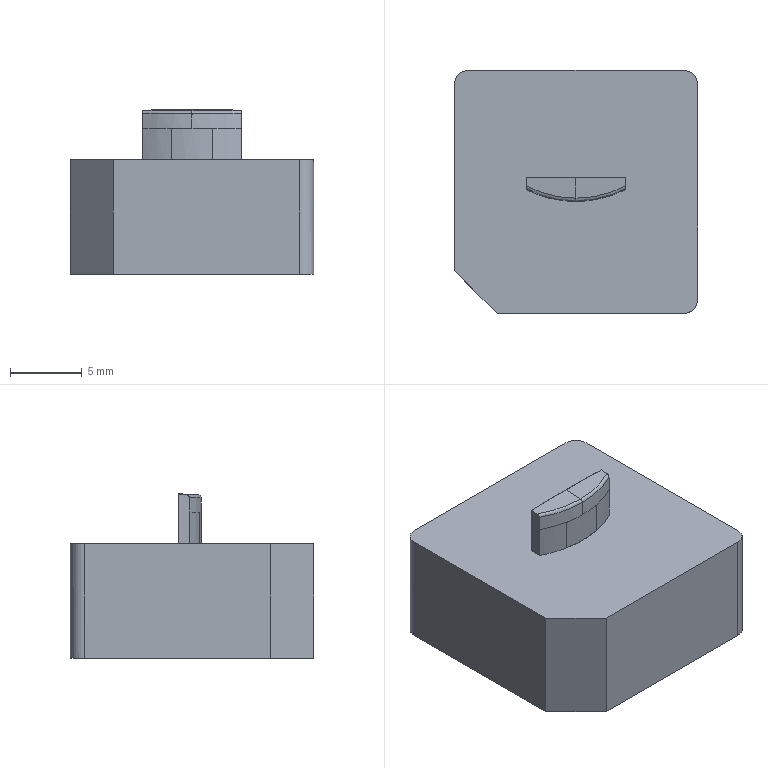CAM job | PowerMill | 3-axis milling, other | part box 17 x 17 x 11.498 mm
Tools:
number,name,type,diameter,tip_radius,length,cutting_length,overhang,flutes,holder,toolpaths_using
1,D10C,end_mill,10.0,0.0,60.0,,30.0,1,D42L35,1
2,D4C_1,end_mill,4.0,0.0,30.0,,4.0,1,D42L35,1
4,R1_1,ball_nosed,2.0,1.0,3.0,,2.0,1,D42L35,1
13,Text_D4_1,taper_spherical,4.0,0.3,60.0,,4.0,1,D42L35,1
1,D10C_1_1,end_mill,10.0,0.0,60.0,,11.96,1,D42L35,3
3,D10_1_1,end_mill,10.0,0.0,60.0,,11.64,1,D42L35,2
10,D3_1_1,end_mill,3.0,0.0,30.0,,3.76,1,D42L35,1
Operations:
program,toolpath,strategy,tool,tool_number,tool_diameter,tip_radius,flutes,spindle_rpm,feed_cut,surface_speed_m_min_computed,feed_per_tooth_computed,tolerance,thickness,stepover,stepdown,cut_length,cut_time_min,total_time_min,workplane
29-B01-8-F,精公开粗01-扫面平行-D10C,raster_area_clear,D10C_1_1,1,10.0,0.0,1.0,8000.0,10000.0,251.33,1.25,0.03,0.28,6.0,1.0,135.36,0.013,0.0178,
29-B01-8-F,精公开粗01-外形偏置-D10C,offset_area_clear,D10C_1_1,1,10.0,0.0,1.0,8000.0,10000.0,251.33,1.25,0.03,0.28,6.0,1.0,1282.164,0.128,0.1524,
29-B01-8-F,精公开粗01-基准台等高-D10C,constantz,D10C_1_1,1,10.0,0.0,1.0,8000.0,10000.0,251.33,1.25,0.03,0.07,5.0,0.4,2129.12,0.213,0.2206,
29-B01-8-F,精公再粗02-外形偏置-D4C,offset_area_clear,D4C_1,2,4.0,0.0,1.0,18000.0,6000.0,226.19,0.3333,0.03,0.0,2.0,1.0,725.851,0.121,0.1322,
29-B01-8-F,精公基准台01-基准面偏置-D10,offset_area_clear,D10_1_1,3,10.0,0.0,1.0,8500.0,600.0,267.04,0.0706,0.005,0.38,5.0,1.0,60.094,0.1,0.1171,
29-B01-8-F,精公基准台01-基准台侧光-D10,profile_area_clear,D10_1_1,3,10.0,0.0,1.0,8500.0,600.0,267.04,0.0706,0.005,0.0,0.08,1.0,193.234,0.322,0.3842,
29-B01-8-F,精公精光01-平行-R1,raster,R1_1,4,2.0,1.0,1.0,18000.0,2000.0,113.1,0.1111,0.005,-0.075,0.03,1.0,712.415,0.356,0.3647,
29-B01-8-F,精公精光02-等高-D3,constantz,D3_1_1,10,3.0,0.0,1.0,18000.0,2000.0,169.65,0.1111,0.005,-0.075,5.0,0.03,2903.178,1.452,1.46,
29-B01-8-F,精公刻字01-刻字-Text_D4,pattern,Text_D4_1,13,4.0,0.3,1.0,15000.0,1000.0,188.5,0.0667,0.005,0.0,5.0,1.0,29.515,0.029,0.0443,
,精公开粗01-外形偏置-D10C_Reference,offset_area_clear,D10C,1,10.0,0.0,1.0,8000.0,10000.0,251.33,1.25,0.03,0.28,6.0,1.0,2421.738,0.242,0.2857,